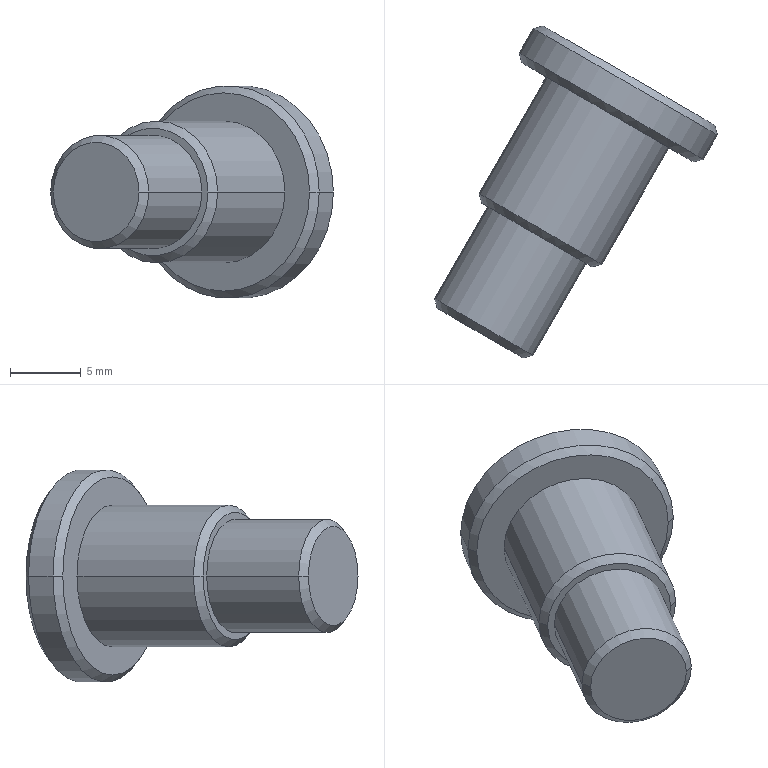Part | SolidWorks | features Chamfer 1, Revolution 1 | 1 solid | 18 faces | box 19.959 x 23.437 x 15 mm | volume 1699 mm3 | cone 8 | cylinder 6 | plane 4 | commonest cylinder face diameters 8 x2 10 x2 15 x2
STEP:
#1=CARTESIAN_POINT('',(-91.294,31.602,0.));
#2=VERTEX_POINT('',#1);
#3=CARTESIAN_POINT('',(-97.356,35.102,0.));
#4=VERTEX_POINT('',#3);
#5=CARTESIAN_POINT('',(-94.325,33.352,0.));
#6=DIRECTION('',(-0.5,-0.866,0.));
#7=DIRECTION('',(-0.866,0.5,0.));
#8=AXIS2_PLACEMENT_3D('',#5,#6,#7);
#9=CIRCLE('',#8,3.5);
#10=EDGE_CURVE('',#2,#4,#9,.T.);
#11=ORIENTED_EDGE('',*,*,#10,.F.);
#12=CARTESIAN_POINT('',(-90.611,31.785,0.));
#13=VERTEX_POINT('',#12);
#14=CARTESIAN_POINT('',(-90.611,31.785,0.));
#15=DIRECTION('',(0.9659,0.2588,0.));
#16=VECTOR('',#15,1000.);
#17=LINE('',#14,#16);
#18=EDGE_CURVE('',#2,#13,#17,.T.);
#19=ORIENTED_EDGE('',*,*,#18,.T.);
#20=CARTESIAN_POINT('',(-97.539,35.785,0.));
#21=VERTEX_POINT('',#20);
#22=CARTESIAN_POINT('',(-94.075,33.785,0.));
#23=DIRECTION('',(0.5,0.866,0.));
#24=DIRECTION('',(-0.866,0.5,0.));
#25=AXIS2_PLACEMENT_3D('',#22,#23,#24);
#26=CIRCLE('',#25,4.);
#27=EDGE_CURVE('',#21,#13,#26,.T.);
#28=ORIENTED_EDGE('',*,*,#27,.F.);
#29=CARTESIAN_POINT('',(-97.539,35.785,0.));
#30=DIRECTION('',(-0.2588,0.9659,0.));
#31=VECTOR('',#30,1000.);
#32=LINE('',#29,#31);
#33=EDGE_CURVE('',#4,#21,#32,.T.);
#34=ORIENTED_EDGE('',*,*,#33,.F.);
#35=EDGE_LOOP('',(#11,#19,#28,#34));
#36=FACE_OUTER_BOUND('',#35,.T.);
#37=CARTESIAN_POINT('',(-94.075,33.785,0.));
#38=DIRECTION('',(0.5,0.866,0.));
#39=DIRECTION('',(-0.866,0.5,0.));
#40=AXIS2_PLACEMENT_3D('',#37,#38,#39);
#41=CONICAL_SURFACE('',#40,4.,0.7854);
#42=ADVANCED_FACE('',(#36),#41,.T.);
#43=CARTESIAN_POINT('',(-86.428,38.031,0.));
#44=VERTEX_POINT('',#43);
#45=CARTESIAN_POINT('',(-94.222,42.531,0.));
#46=VERTEX_POINT('',#45);
#47=CARTESIAN_POINT('',(-90.325,40.281,0.));
#48=DIRECTION('',(-0.5,-0.866,0.));
#49=DIRECTION('',(-0.866,0.5,0.));
#50=AXIS2_PLACEMENT_3D('',#47,#48,#49);
#51=CIRCLE('',#50,4.5);
#52=EDGE_CURVE('',#44,#46,#51,.T.);
#53=ORIENTED_EDGE('',*,*,#52,.F.);
#54=CARTESIAN_POINT('',(-85.745,38.214,0.));
#55=VERTEX_POINT('',#54);
#56=CARTESIAN_POINT('',(-85.745,38.214,0.));
#57=DIRECTION('',(0.9659,0.2588,0.));
#58=VECTOR('',#57,1000.);
#59=LINE('',#56,#58);
#60=EDGE_CURVE('',#44,#55,#59,.T.);
#61=ORIENTED_EDGE('',*,*,#60,.T.);
#62=CARTESIAN_POINT('',(-94.405,43.214,0.));
#63=VERTEX_POINT('',#62);
#64=CARTESIAN_POINT('',(-90.075,40.714,0.));
#65=DIRECTION('',(0.5,0.866,0.));
#66=DIRECTION('',(-0.866,0.5,0.));
#67=AXIS2_PLACEMENT_3D('',#64,#65,#66);
#68=CIRCLE('',#67,5.);
#69=EDGE_CURVE('',#63,#55,#68,.T.);
#70=ORIENTED_EDGE('',*,*,#69,.F.);
#71=CARTESIAN_POINT('',(-94.405,43.214,0.));
#72=DIRECTION('',(-0.2588,0.9659,0.));
#73=VECTOR('',#72,1000.);
#74=LINE('',#71,#73);
#75=EDGE_CURVE('',#46,#63,#74,.T.);
#76=ORIENTED_EDGE('',*,*,#75,.F.);
#77=EDGE_LOOP('',(#53,#61,#70,#76));
#78=FACE_OUTER_BOUND('',#77,.T.);
#79=CARTESIAN_POINT('',(-90.075,40.714,0.));
#80=DIRECTION('',(0.5,0.866,0.));
#81=DIRECTION('',(-0.866,0.5,0.));
#82=AXIS2_PLACEMENT_3D('',#79,#80,#81);
#83=CONICAL_SURFACE('',#82,5.,0.7854);
#84=ADVANCED_FACE('',(#78),#83,.T.);
#85=CARTESIAN_POINT('',(-79.263,45.441,0.));
#86=VERTEX_POINT('',#85);
#87=CARTESIAN_POINT('',(-91.387,52.441,0.));
#88=VERTEX_POINT('',#87);
#89=CARTESIAN_POINT('',(-85.325,48.941,0.));
#90=DIRECTION('',(-0.5,-0.866,0.));
#91=DIRECTION('',(-0.866,0.5,0.));
#92=AXIS2_PLACEMENT_3D('',#89,#90,#91);
#93=CIRCLE('',#92,7.);
#94=EDGE_CURVE('',#86,#88,#93,.T.);
#95=ORIENTED_EDGE('',*,*,#94,.F.);
#96=CARTESIAN_POINT('',(-78.58,45.624,0.));
#97=VERTEX_POINT('',#96);
#98=CARTESIAN_POINT('',(-78.58,45.624,0.));
#99=DIRECTION('',(0.9659,0.2588,0.));
#100=VECTOR('',#99,1000.);
#101=LINE('',#98,#100);
#102=EDGE_CURVE('',#86,#97,#101,.T.);
#103=ORIENTED_EDGE('',*,*,#102,.T.);
#104=CARTESIAN_POINT('',(-91.57,53.124,0.));
#105=VERTEX_POINT('',#104);
#106=CARTESIAN_POINT('',(-85.075,49.374,0.));
#107=DIRECTION('',(0.5,0.866,0.));
#108=DIRECTION('',(-0.866,0.5,0.));
#109=AXIS2_PLACEMENT_3D('',#106,#107,#108);
#110=CIRCLE('',#109,7.5);
#111=EDGE_CURVE('',#105,#97,#110,.T.);
#112=ORIENTED_EDGE('',*,*,#111,.F.);
#113=CARTESIAN_POINT('',(-91.57,53.124,0.));
#114=DIRECTION('',(-0.2588,0.9659,0.));
#115=VECTOR('',#114,1000.);
#116=LINE('',#113,#115);
#117=EDGE_CURVE('',#88,#105,#116,.T.);
#118=ORIENTED_EDGE('',*,*,#117,.F.);
#119=EDGE_LOOP('',(#95,#103,#112,#118));
#120=FACE_OUTER_BOUND('',#119,.T.);
#121=CARTESIAN_POINT('',(-85.075,49.374,0.));
#122=DIRECTION('',(0.5,0.866,0.));
#123=DIRECTION('',(-0.866,0.5,0.));
#124=AXIS2_PLACEMENT_3D('',#121,#122,#123);
#125=CONICAL_SURFACE('',#124,7.5,0.7854);
#126=ADVANCED_FACE('',(#120),#125,.T.);
#127=CARTESIAN_POINT('',(-89.887,55.039,0.));
#128=VERTEX_POINT('',#127);
#129=CARTESIAN_POINT('',(-77.763,48.039,0.));
#130=VERTEX_POINT('',#129);
#131=CARTESIAN_POINT('',(-83.825,51.539,0.));
#132=DIRECTION('',(0.5,0.866,0.));
#133=DIRECTION('',(0.866,-0.5,0.));
#134=AXIS2_PLACEMENT_3D('',#131,#132,#133);
#135=CIRCLE('',#134,7.);
#136=EDGE_CURVE('',#128,#130,#135,.T.);
#137=ORIENTED_EDGE('',*,*,#136,.F.);
#138=CARTESIAN_POINT('',(-90.57,54.856,0.));
#139=VERTEX_POINT('',#138);
#140=CARTESIAN_POINT('',(-89.887,55.039,0.));
#141=DIRECTION('',(-0.9659,-0.2588,0.));
#142=VECTOR('',#141,1000.);
#143=LINE('',#140,#142);
#144=EDGE_CURVE('',#128,#139,#143,.T.);
#145=ORIENTED_EDGE('',*,*,#144,.T.);
#146=CARTESIAN_POINT('',(-77.58,47.356,0.));
#147=VERTEX_POINT('',#146);
#148=CARTESIAN_POINT('',(-84.075,51.106,0.));
#149=DIRECTION('',(-0.5,-0.866,0.));
#150=DIRECTION('',(0.866,-0.5,0.));
#151=AXIS2_PLACEMENT_3D('',#148,#149,#150);
#152=CIRCLE('',#151,7.5);
#153=EDGE_CURVE('',#147,#139,#152,.T.);
#154=ORIENTED_EDGE('',*,*,#153,.F.);
#155=CARTESIAN_POINT('',(-77.763,48.039,0.));
#156=DIRECTION('',(0.2588,-0.9659,0.));
#157=VECTOR('',#156,1000.);
#158=LINE('',#155,#157);
#159=EDGE_CURVE('',#130,#147,#158,.T.);
#160=ORIENTED_EDGE('',*,*,#159,.F.);
#161=EDGE_LOOP('',(#137,#145,#154,#160));
#162=FACE_OUTER_BOUND('',#161,.T.);
#163=CARTESIAN_POINT('',(-83.825,51.539,0.));
#164=DIRECTION('',(-0.5,-0.866,0.));
#165=DIRECTION('',(0.866,-0.5,0.));
#166=AXIS2_PLACEMENT_3D('',#163,#164,#165);
#167=CONICAL_SURFACE('',#166,7.,0.7854);
#168=ADVANCED_FACE('',(#162),#167,.T.);
#169=ORIENTED_EDGE('',*,*,#27,.T.);
#170=CARTESIAN_POINT('',(-86.861,38.281,0.));
#171=VERTEX_POINT('',#170);
#172=CARTESIAN_POINT('',(-80.361,49.539,0.));
#173=DIRECTION('',(0.5,0.866,0.));
#174=VECTOR('',#173,1000.);
#175=LINE('',#172,#174);
#176=EDGE_CURVE('',#13,#171,#175,.T.);
#177=ORIENTED_EDGE('',*,*,#176,.T.);
#178=CARTESIAN_POINT('',(-93.789,42.281,0.));
#179=VERTEX_POINT('',#178);
#180=CARTESIAN_POINT('',(-90.325,40.281,0.));
#181=DIRECTION('',(0.5,0.866,0.));
#182=DIRECTION('',(-0.866,0.5,0.));
#183=AXIS2_PLACEMENT_3D('',#180,#181,#182);
#184=CIRCLE('',#183,4.);
#185=EDGE_CURVE('',#179,#171,#184,.T.);
#186=ORIENTED_EDGE('',*,*,#185,.F.);
#187=CARTESIAN_POINT('',(-87.289,53.539,0.));
#188=DIRECTION('',(0.5,0.866,0.));
#189=VECTOR('',#188,1000.);
#190=LINE('',#187,#189);
#191=EDGE_CURVE('',#21,#179,#190,.T.);
#192=ORIENTED_EDGE('',*,*,#191,.F.);
#193=EDGE_LOOP('',(#169,#177,#186,#192));
#194=FACE_OUTER_BOUND('',#193,.T.);
#195=CARTESIAN_POINT('',(-83.825,51.539,0.));
#196=DIRECTION('',(0.5,0.866,0.));
#197=DIRECTION('',(-0.866,0.5,0.));
#198=AXIS2_PLACEMENT_3D('',#195,#196,#197);
#199=CYLINDRICAL_SURFACE('',#198,4.);
#200=ADVANCED_FACE('',(#194),#199,.T.);
#201=ORIENTED_EDGE('',*,*,#111,.T.);
#202=CARTESIAN_POINT('',(-77.33,47.789,0.));
#203=DIRECTION('',(0.5,0.866,0.));
#204=VECTOR('',#203,1000.);
#205=LINE('',#202,#204);
#206=EDGE_CURVE('',#97,#147,#205,.T.);
#207=ORIENTED_EDGE('',*,*,#206,.T.);
#208=ORIENTED_EDGE('',*,*,#153,.T.);
#209=CARTESIAN_POINT('',(-90.32,55.289,0.));
#210=DIRECTION('',(0.5,0.866,0.));
#211=VECTOR('',#210,1000.);
#212=LINE('',#209,#211);
#213=EDGE_CURVE('',#105,#139,#212,.T.);
#214=ORIENTED_EDGE('',*,*,#213,.F.);
#215=EDGE_LOOP('',(#201,#207,#208,#214));
#216=FACE_OUTER_BOUND('',#215,.T.);
#217=CARTESIAN_POINT('',(-83.825,51.539,0.));
#218=DIRECTION('',(0.5,0.866,0.));
#219=DIRECTION('',(-0.866,0.5,0.));
#220=AXIS2_PLACEMENT_3D('',#217,#218,#219);
#221=CYLINDRICAL_SURFACE('',#220,7.5);
#222=ADVANCED_FACE('',(#216),#221,.T.);
#223=ORIENTED_EDGE('',*,*,#69,.T.);
#224=CARTESIAN_POINT('',(-80.995,46.441,0.));
#225=VERTEX_POINT('',#224);
#226=CARTESIAN_POINT('',(-79.495,49.039,0.));
#227=DIRECTION('',(0.5,0.866,0.));
#228=VECTOR('',#227,1000.);
#229=LINE('',#226,#228);
#230=EDGE_CURVE('',#55,#225,#229,.T.);
#231=ORIENTED_EDGE('',*,*,#230,.T.);
#232=CARTESIAN_POINT('',(-89.655,51.441,0.));
#233=VERTEX_POINT('',#232);
#234=CARTESIAN_POINT('',(-85.325,48.941,0.));
#235=DIRECTION('',(0.5,0.866,0.));
#236=DIRECTION('',(-0.866,0.5,0.));
#237=AXIS2_PLACEMENT_3D('',#234,#235,#236);
#238=CIRCLE('',#237,5.);
#239=EDGE_CURVE('',#233,#225,#238,.T.);
#240=ORIENTED_EDGE('',*,*,#239,.F.);
#241=CARTESIAN_POINT('',(-88.155,54.039,0.));
#242=DIRECTION('',(0.5,0.866,0.));
#243=VECTOR('',#242,1000.);
#244=LINE('',#241,#243);
#245=EDGE_CURVE('',#63,#233,#244,.T.);
#246=ORIENTED_EDGE('',*,*,#245,.F.);
#247=EDGE_LOOP('',(#223,#231,#240,#246));
#248=FACE_OUTER_BOUND('',#247,.T.);
#249=CARTESIAN_POINT('',(-83.825,51.539,0.));
#250=DIRECTION('',(0.5,0.866,0.));
#251=DIRECTION('',(-0.866,0.5,0.));
#252=AXIS2_PLACEMENT_3D('',#249,#250,#251);
#253=CYLINDRICAL_SURFACE('',#252,5.);
#254=ADVANCED_FACE('',(#248),#253,.T.);
#255=CARTESIAN_POINT('',(-90.325,40.281,0.));
#256=DIRECTION('',(-0.5,-0.866,0.));
#257=DIRECTION('',(-0.866,0.5,0.));
#258=AXIS2_PLACEMENT_3D('',#255,#256,#257);
#259=CIRCLE('',#258,4.5);
#260=EDGE_CURVE('',#46,#44,#259,.T.);
#261=ORIENTED_EDGE('',*,*,#260,.T.);
#262=ORIENTED_EDGE('',*,*,#52,.T.);
#263=EDGE_LOOP('',(#261,#262));
#264=FACE_OUTER_BOUND('',#263,.T.);
#265=ORIENTED_EDGE('',*,*,#185,.T.);
#266=CARTESIAN_POINT('',(-90.325,40.281,0.));
#267=DIRECTION('',(0.5,0.866,0.));
#268=DIRECTION('',(-0.866,0.5,0.));
#269=AXIS2_PLACEMENT_3D('',#266,#267,#268);
#270=CIRCLE('',#269,4.);
#271=EDGE_CURVE('',#171,#179,#270,.T.);
#272=ORIENTED_EDGE('',*,*,#271,.T.);
#273=EDGE_LOOP('',(#265,#272));
#274=FACE_BOUND('',#273,.T.);
#275=CARTESIAN_POINT('',(-85.995,37.781,0.));
#276=DIRECTION('',(0.5,0.866,0.));
#277=DIRECTION('',(-0.866,0.5,0.));
#278=AXIS2_PLACEMENT_3D('',#275,#276,#277);
#279=PLANE('',#278);
#280=ADVANCED_FACE('',(#264,#274),#279,.F.);
#281=ORIENTED_EDGE('',*,*,#230,.F.);
#282=CARTESIAN_POINT('',(-90.075,40.714,0.));
#283=DIRECTION('',(0.5,0.866,0.));
#284=DIRECTION('',(-0.866,0.5,0.));
#285=AXIS2_PLACEMENT_3D('',#282,#283,#284);
#286=CIRCLE('',#285,5.);
#287=EDGE_CURVE('',#55,#63,#286,.T.);
#288=ORIENTED_EDGE('',*,*,#287,.T.);
#289=ORIENTED_EDGE('',*,*,#245,.T.);
#290=CARTESIAN_POINT('',(-85.325,48.941,0.));
#291=DIRECTION('',(0.5,0.866,0.));
#292=DIRECTION('',(-0.866,0.5,0.));
#293=AXIS2_PLACEMENT_3D('',#290,#291,#292);
#294=CIRCLE('',#293,5.);
#295=EDGE_CURVE('',#225,#233,#294,.T.);
#296=ORIENTED_EDGE('',*,*,#295,.F.);
#297=EDGE_LOOP('',(#281,#288,#289,#296));
#298=FACE_OUTER_BOUND('',#297,.T.);
#299=CARTESIAN_POINT('',(-83.825,51.539,0.));
#300=DIRECTION('',(0.5,0.866,0.));
#301=DIRECTION('',(-0.866,0.5,0.));
#302=AXIS2_PLACEMENT_3D('',#299,#300,#301);
#303=CYLINDRICAL_SURFACE('',#302,5.);
#304=ADVANCED_FACE('',(#298),#303,.T.);
#305=CARTESIAN_POINT('',(-85.325,48.941,0.));
#306=DIRECTION('',(-0.5,-0.866,0.));
#307=DIRECTION('',(-0.866,0.5,0.));
#308=AXIS2_PLACEMENT_3D('',#305,#306,#307);
#309=CIRCLE('',#308,7.);
#310=EDGE_CURVE('',#88,#86,#309,.T.);
#311=ORIENTED_EDGE('',*,*,#310,.T.);
#312=ORIENTED_EDGE('',*,*,#94,.T.);
#313=EDGE_LOOP('',(#311,#312));
#314=FACE_OUTER_BOUND('',#313,.T.);
#315=ORIENTED_EDGE('',*,*,#239,.T.);
#316=ORIENTED_EDGE('',*,*,#295,.T.);
#317=EDGE_LOOP('',(#315,#316));
#318=FACE_BOUND('',#317,.T.);
#319=CARTESIAN_POINT('',(-80.995,46.441,0.));
#320=DIRECTION('',(0.5,0.866,0.));
#321=DIRECTION('',(-0.866,0.5,0.));
#322=AXIS2_PLACEMENT_3D('',#319,#320,#321);
#323=PLANE('',#322);
#324=ADVANCED_FACE('',(#314,#318),#323,.F.);
#325=ORIENTED_EDGE('',*,*,#206,.F.);
#326=CARTESIAN_POINT('',(-85.075,49.374,0.));
#327=DIRECTION('',(0.5,0.866,0.));
#328=DIRECTION('',(-0.866,0.5,0.));
#329=AXIS2_PLACEMENT_3D('',#326,#327,#328);
#330=CIRCLE('',#329,7.5);
#331=EDGE_CURVE('',#97,#105,#330,.T.);
#332=ORIENTED_EDGE('',*,*,#331,.T.);
#333=ORIENTED_EDGE('',*,*,#213,.T.);
#334=CARTESIAN_POINT('',(-84.075,51.106,0.));
#335=DIRECTION('',(-0.5,-0.866,0.));
#336=DIRECTION('',(0.866,-0.5,0.));
#337=AXIS2_PLACEMENT_3D('',#334,#335,#336);
#338=CIRCLE('',#337,7.5);
#339=EDGE_CURVE('',#139,#147,#338,.T.);
#340=ORIENTED_EDGE('',*,*,#339,.T.);
#341=EDGE_LOOP('',(#325,#332,#333,#340));
#342=FACE_OUTER_BOUND('',#341,.T.);
#343=CARTESIAN_POINT('',(-83.825,51.539,0.));
#344=DIRECTION('',(0.5,0.866,0.));
#345=DIRECTION('',(-0.866,0.5,0.));
#346=AXIS2_PLACEMENT_3D('',#343,#344,#345);
#347=CYLINDRICAL_SURFACE('',#346,7.5);
#348=ADVANCED_FACE('',(#342),#347,.T.);
#349=CARTESIAN_POINT('',(-83.825,51.539,0.));
#350=DIRECTION('',(0.5,0.866,0.));
#351=DIRECTION('',(0.866,-0.5,0.));
#352=AXIS2_PLACEMENT_3D('',#349,#350,#351);
#353=CIRCLE('',#352,7.);
#354=EDGE_CURVE('',#130,#128,#353,.T.);
#355=ORIENTED_EDGE('',*,*,#354,.T.);
#356=ORIENTED_EDGE('',*,*,#136,.T.);
#357=EDGE_LOOP('',(#355,#356));
#358=FACE_OUTER_BOUND('',#357,.T.);
#359=CARTESIAN_POINT('',(-77.33,47.789,0.));
#360=DIRECTION('',(-0.5,-0.866,0.));
#361=DIRECTION('',(0.866,-0.5,0.));
#362=AXIS2_PLACEMENT_3D('',#359,#360,#361);
#363=PLANE('',#362);
#364=ADVANCED_FACE('',(#358),#363,.F.);
#365=CARTESIAN_POINT('',(-94.325,33.352,0.));
#366=DIRECTION('',(-0.5,-0.866,0.));
#367=DIRECTION('',(-0.866,0.5,0.));
#368=AXIS2_PLACEMENT_3D('',#365,#366,#367);
#369=CIRCLE('',#368,3.5);
#370=EDGE_CURVE('',#4,#2,#369,.T.);
#371=ORIENTED_EDGE('',*,*,#370,.T.);
#372=ORIENTED_EDGE('',*,*,#10,.T.);
#373=EDGE_LOOP('',(#371,#372));
#374=FACE_OUTER_BOUND('',#373,.T.);
#375=CARTESIAN_POINT('',(-90.861,31.352,0.));
#376=DIRECTION('',(0.5,0.866,0.));
#377=DIRECTION('',(-0.866,0.5,0.));
#378=AXIS2_PLACEMENT_3D('',#375,#376,#377);
#379=PLANE('',#378);
#380=ADVANCED_FACE('',(#374),#379,.F.);
#381=ORIENTED_EDGE('',*,*,#176,.F.);
#382=CARTESIAN_POINT('',(-94.075,33.785,0.));
#383=DIRECTION('',(0.5,0.866,0.));
#384=DIRECTION('',(-0.866,0.5,0.));
#385=AXIS2_PLACEMENT_3D('',#382,#383,#384);
#386=CIRCLE('',#385,4.);
#387=EDGE_CURVE('',#13,#21,#386,.T.);
#388=ORIENTED_EDGE('',*,*,#387,.T.);
#389=ORIENTED_EDGE('',*,*,#191,.T.);
#390=ORIENTED_EDGE('',*,*,#271,.F.);
#391=EDGE_LOOP('',(#381,#388,#389,#390));
#392=FACE_OUTER_BOUND('',#391,.T.);
#393=CARTESIAN_POINT('',(-83.825,51.539,0.));
#394=DIRECTION('',(0.5,0.866,0.));
#395=DIRECTION('',(-0.866,0.5,0.));
#396=AXIS2_PLACEMENT_3D('',#393,#394,#395);
#397=CYLINDRICAL_SURFACE('',#396,4.);
#398=ADVANCED_FACE('',(#392),#397,.T.);
#399=ORIENTED_EDGE('',*,*,#144,.F.);
#400=ORIENTED_EDGE('',*,*,#354,.F.);
#401=ORIENTED_EDGE('',*,*,#159,.T.);
#402=ORIENTED_EDGE('',*,*,#339,.F.);
#403=EDGE_LOOP('',(#399,#400,#401,#402));
#404=FACE_OUTER_BOUND('',#403,.T.);
#405=CARTESIAN_POINT('',(-83.825,51.539,0.));
#406=DIRECTION('',(-0.5,-0.866,0.));
#407=DIRECTION('',(0.866,-0.5,0.));
#408=AXIS2_PLACEMENT_3D('',#405,#406,#407);
#409=CONICAL_SURFACE('',#408,7.,0.7854);
#410=ADVANCED_FACE('',(#404),#409,.T.);
#411=ORIENTED_EDGE('',*,*,#102,.F.);
#412=ORIENTED_EDGE('',*,*,#310,.F.);
#413=ORIENTED_EDGE('',*,*,#117,.T.);
#414=ORIENTED_EDGE('',*,*,#331,.F.);
#415=EDGE_LOOP('',(#411,#412,#413,#414));
#416=FACE_OUTER_BOUND('',#415,.T.);
#417=CARTESIAN_POINT('',(-85.075,49.374,0.));
#418=DIRECTION('',(0.5,0.866,0.));
#419=DIRECTION('',(-0.866,0.5,0.));
#420=AXIS2_PLACEMENT_3D('',#417,#418,#419);
#421=CONICAL_SURFACE('',#420,7.5,0.7854);
#422=ADVANCED_FACE('',(#416),#421,.T.);
#423=ORIENTED_EDGE('',*,*,#60,.F.);
#424=ORIENTED_EDGE('',*,*,#260,.F.);
#425=ORIENTED_EDGE('',*,*,#75,.T.);
#426=ORIENTED_EDGE('',*,*,#287,.F.);
#427=EDGE_LOOP('',(#423,#424,#425,#426));
#428=FACE_OUTER_BOUND('',#427,.T.);
#429=CARTESIAN_POINT('',(-90.075,40.714,0.));
#430=DIRECTION('',(0.5,0.866,0.));
#431=DIRECTION('',(-0.866,0.5,0.));
#432=AXIS2_PLACEMENT_3D('',#429,#430,#431);
#433=CONICAL_SURFACE('',#432,5.,0.7854);
#434=ADVANCED_FACE('',(#428),#433,.T.);
#435=ORIENTED_EDGE('',*,*,#18,.F.);
#436=ORIENTED_EDGE('',*,*,#370,.F.);
#437=ORIENTED_EDGE('',*,*,#33,.T.);
#438=ORIENTED_EDGE('',*,*,#387,.F.);
#439=EDGE_LOOP('',(#435,#436,#437,#438));
#440=FACE_OUTER_BOUND('',#439,.T.);
#441=CARTESIAN_POINT('',(-94.075,33.785,0.));
#442=DIRECTION('',(0.5,0.866,0.));
#443=DIRECTION('',(-0.866,0.5,0.));
#444=AXIS2_PLACEMENT_3D('',#441,#442,#443);
#445=CONICAL_SURFACE('',#444,4.,0.7854);
#446=ADVANCED_FACE('',(#440),#445,.T.);
#447=CLOSED_SHELL('',(#42,#84,#126,#168,#200,#222,#254,#280,#304,#324,#348,#364,#380,#398,#410,#422,#434,#446));
#448=MANIFOLD_SOLID_BREP('',#447);
#449=CARTESIAN_POINT('',(0.,0.,0.));
#450=DIRECTION('',(0.,0.,1.));
#451=DIRECTION('',(1.,0.,0.));
#452=AXIS2_PLACEMENT_3D('',#449,#450,#451);
#453=(LENGTH_UNIT()NAMED_UNIT(*)SI_UNIT(.MILLI.,.METRE.));
#454=UNCERTAINTY_MEASURE_WITH_UNIT(LENGTH_MEASURE(0.00001),#453,'','');
#455=(NAMED_UNIT(*)PLANE_ANGLE_UNIT()SI_UNIT($,.RADIAN.));
#456=(NAMED_UNIT(*)SI_UNIT($,.STERADIAN.)SOLID_ANGLE_UNIT());
#457=(GEOMETRIC_REPRESENTATION_CONTEXT(3)GLOBAL_UNCERTAINTY_ASSIGNED_CONTEXT((#454))GLOBAL_UNIT_ASSIGNED_CONTEXT((#453,#455,#456))REPRESENTATION_CONTEXT('',''));
#458=ADVANCED_BREP_SHAPE_REPRESENTATION('',(#448,#452),#457);